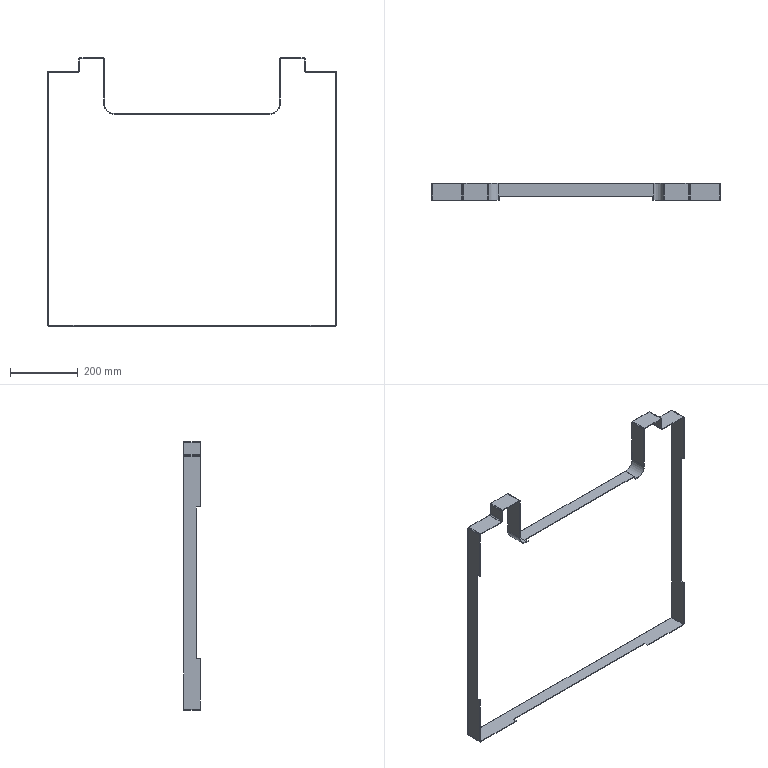Part | SolidWorks | features ICE 7, Fillet 5, Extrusion 1, Shell 1 | 1 solid | 65 faces | box 851 x 50 x 791 mm | volume 311497 mm3 | plane 41 | cylinder 24 | commonest cylinder face diameters 6 x10 2 x8 10 x2 56 x2 60 x2